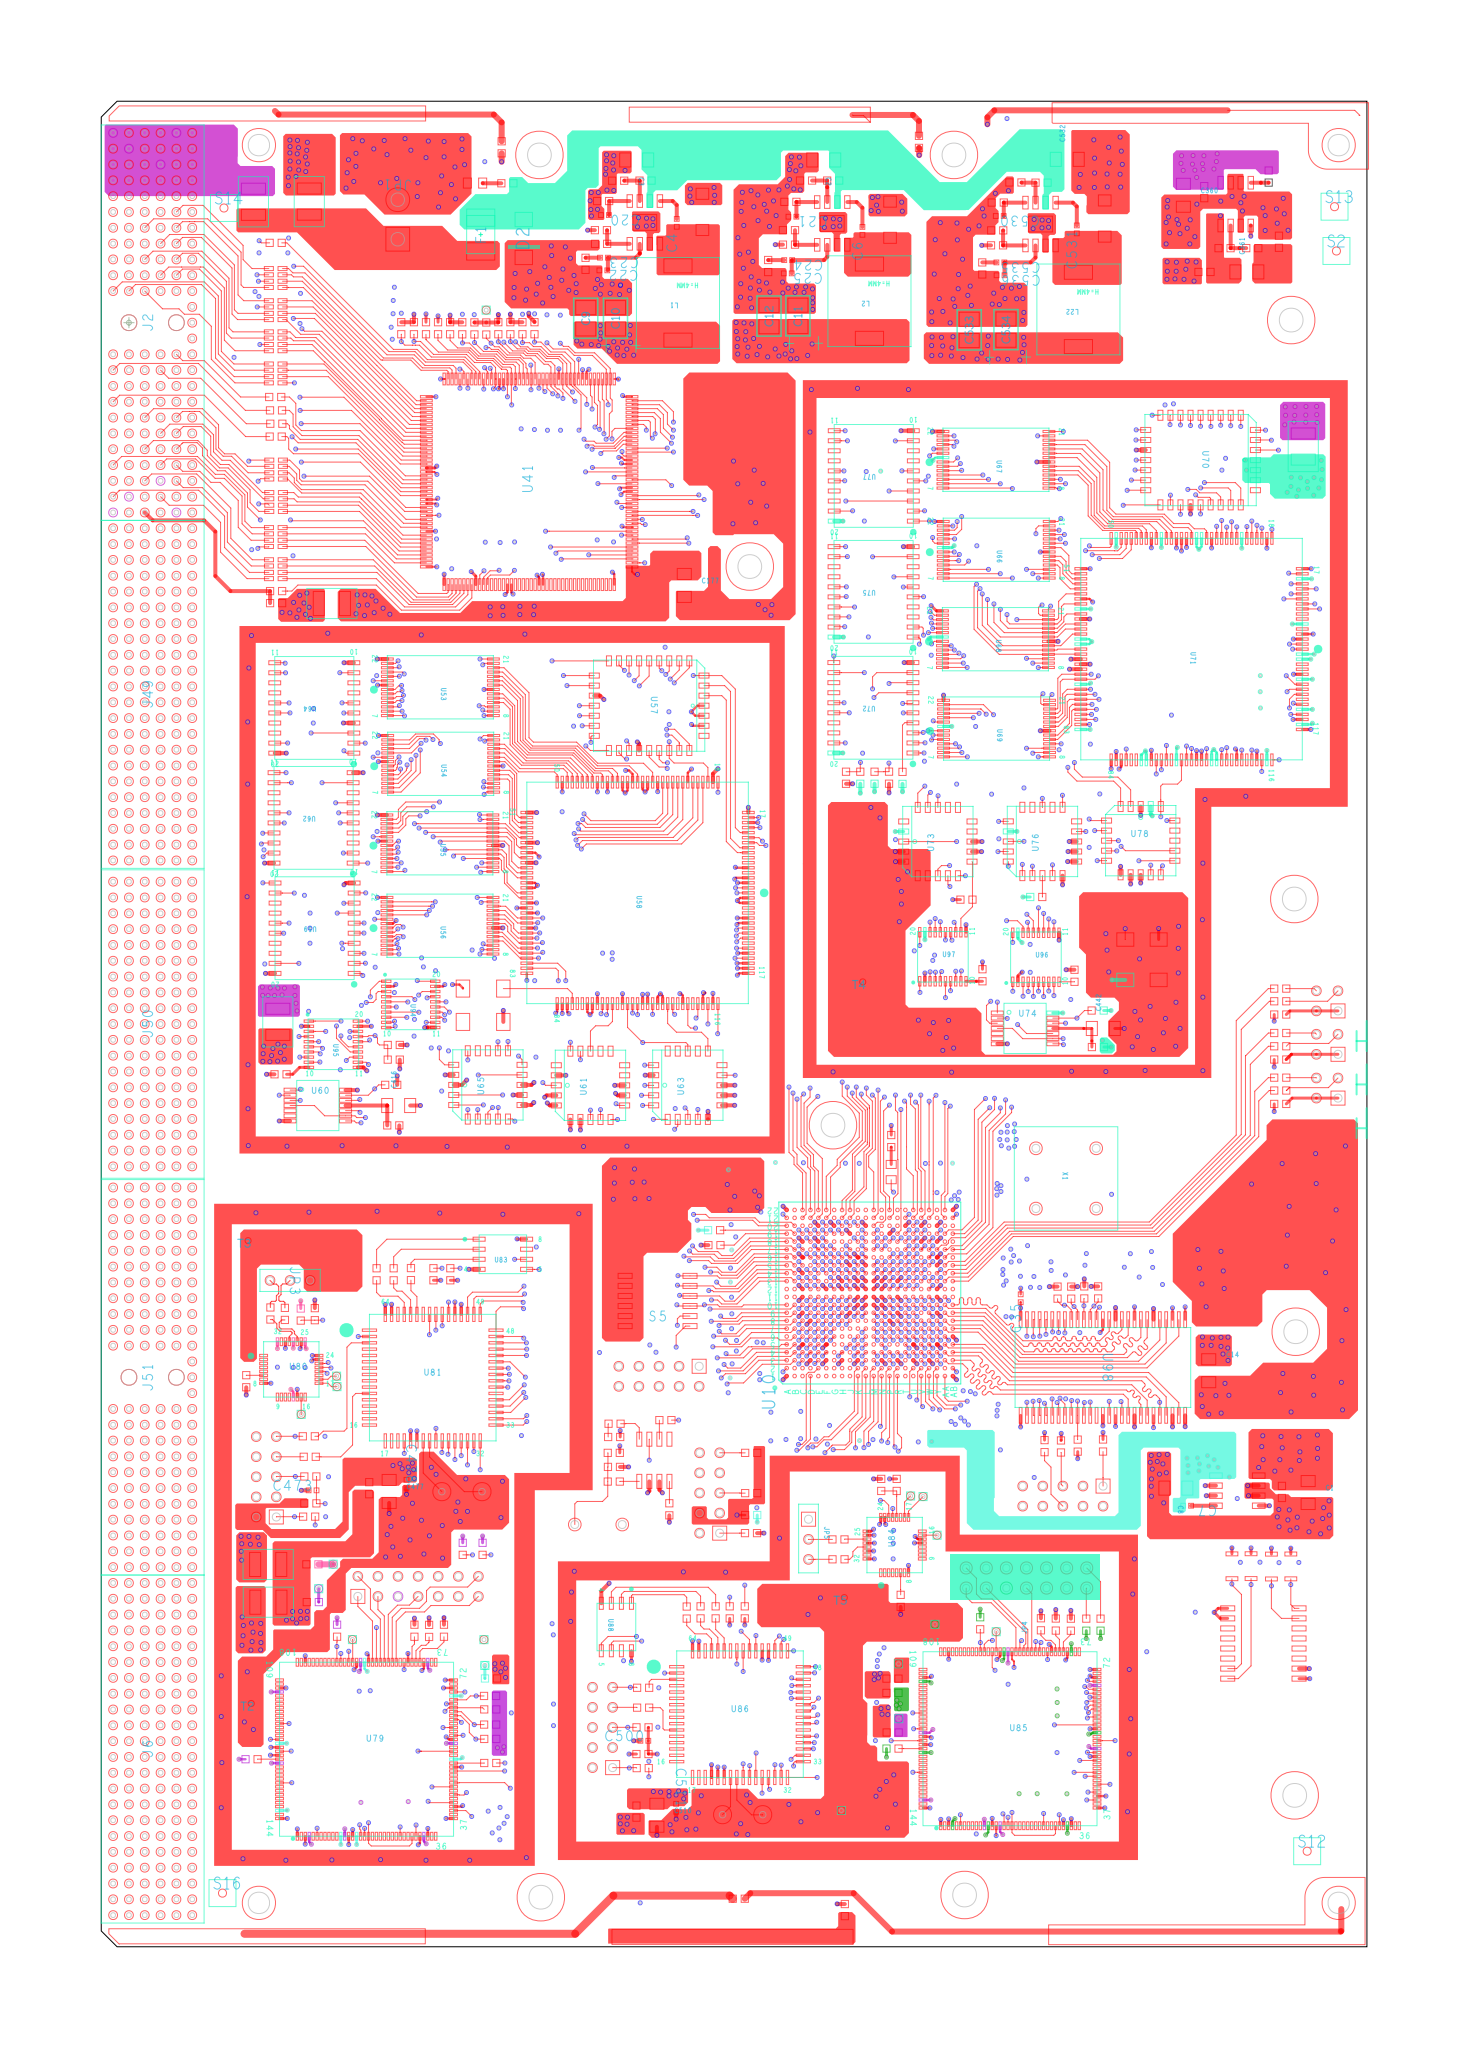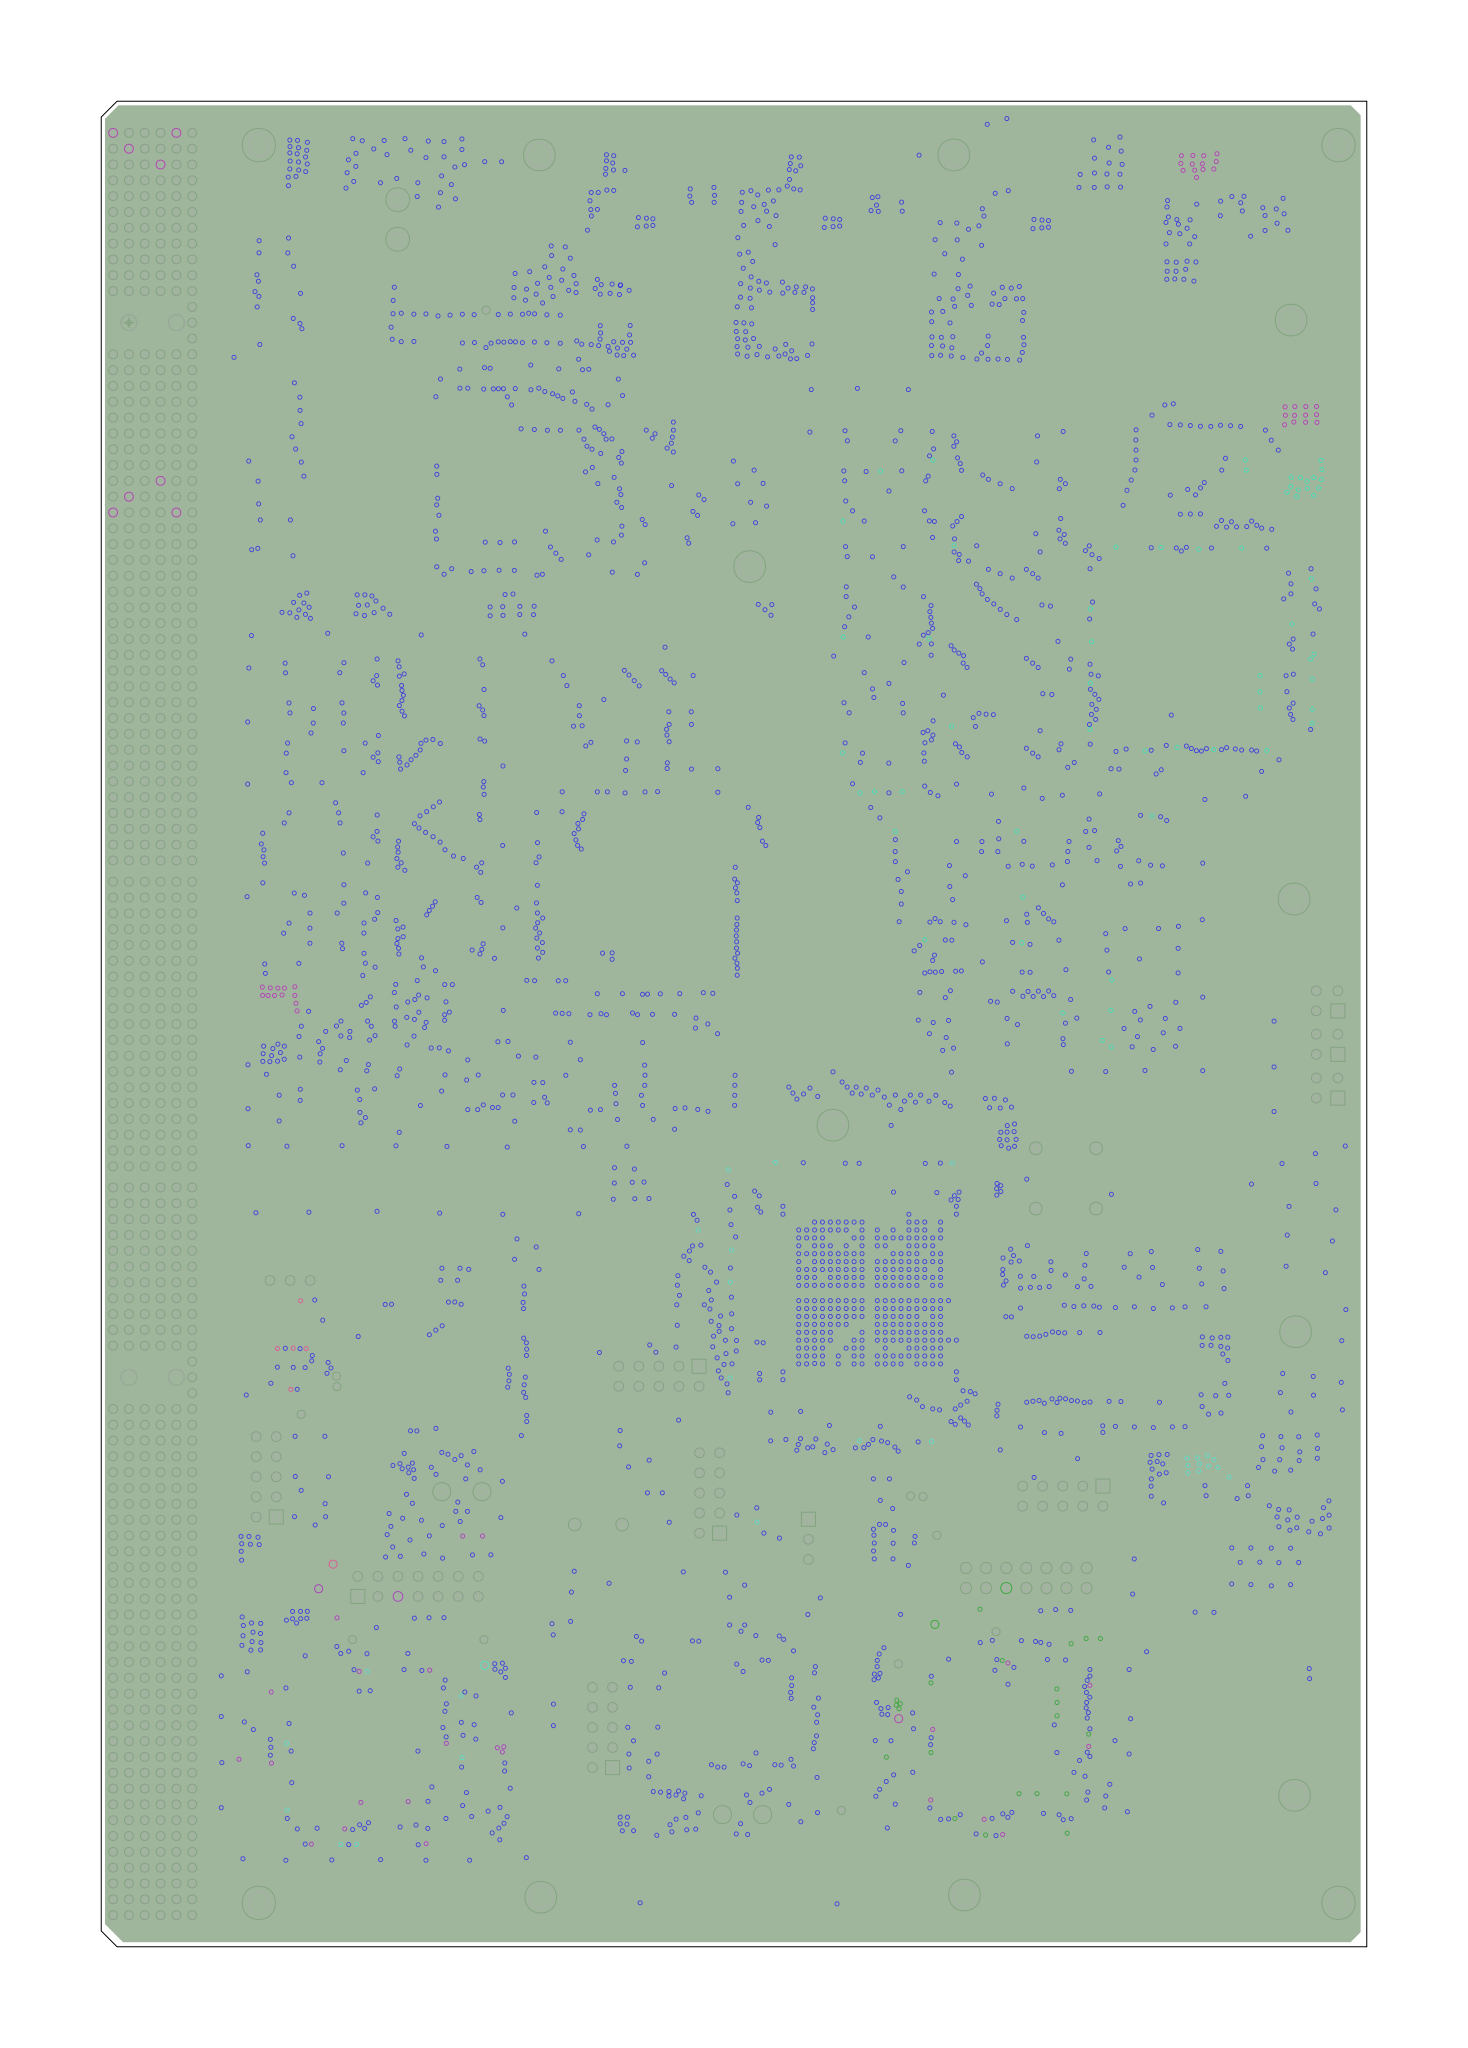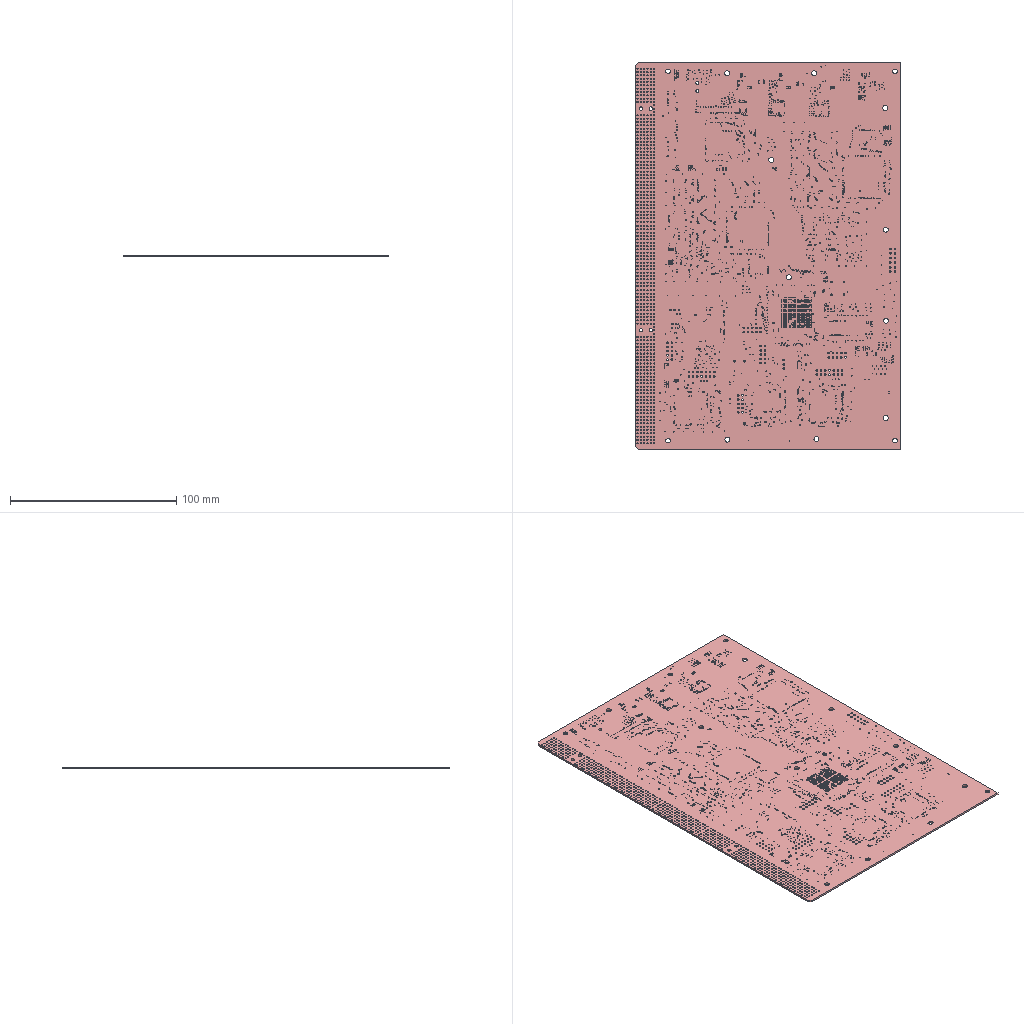Circuit board layout | Cadence Allegro | box 160 x 233.4 x 1.1 mm
Layer stack:
# Cadence Allegro layer stack of  (unit mm; from the constraint file cross-section; dielectric type: 0 not recorded (Allegro does not mark core vs prepreg), 3 surface material)
index,name,kind,layer,copper_thickness_mm,dielectric_type,dielectric_thickness_mm,dielectric_material,dielectric_constant
0,Top Surface,other,,,,,,
1,TOP,copper,TOP,0.0483,,,,
2,Dielectric1,dielectric,,,0,0.1143,FR-4,4.5
3,GND2,copper,GND2,0.0305,,,,
4,Dielectric2,dielectric,,,0,0.254,FR-4,4.5
5,IN3,copper,IN3,0.0305,,,,
6,Dielectric3,dielectric,,,0,0.254,FR-4,4.5
7,IN4,copper,IN4,0.0305,,,,
8,Dielectric4,dielectric,,,0,0.254,FR-4,4.5
9,VCC5,copper,VCC5,0.0305,,,,
10,Dielectric5,dielectric,,,0,0.1143,FR-4,4.5
11,BOTTOM,copper,BOTTOM,0.0483,,,,
12,Bottom Surface,other,,,,,,
# drill layer pairs: low layer,high layer
drill_pair,TOP,BOTTOM
Part placement, first 524 of 690 lines:
REFDES,COMP_VALUE,SYM_NAME,SYM_X,SYM_Y,SYM_ROTATE,SYM_MIRROR
C1,10uF,16V,CP3216,5868.969,-5823.437,0.000,NO
C2,10uF,16V,CP3216,3458.000,810.000,270.000,NO
C3,10uF,16V,CP3216,2527.000,810.000,270.000,NO
C4,0.1uF,C0402,2726.500,497.000,90.000,NO
C5,0.1uF,C0402,4890.500,-4389.500,90.000,YES
C6,0.1uF,C0402,3650.500,457.000,90.000,NO
C7,0.1uF,C0402,5266.508,-5889.256,180.000,NO
C8,10uF,16V,CP3216,5210.500,-5801.500,270.000,NO
C9,47uF,CP3528,2273.500,22.000,180.000,NO
C10,47uF,CP3528,2421.500,22.000,180.000,NO
C11,47uF,CP3528,3329.500,34.000,180.000,NO
C12,47uF,CP3528,3185.500,33.000,180.000,NO
C14,10uF,16V,CP3216,5374.000,-5160.000,0.000,NO
C15,10uF,16V,CP3216,4272.000,-5367.000,0.000,YES
C16,0.1uF,C0402,4953.992,-4654.256,270.000,YES
C17,0.1uF,C0402,2616.500,-5791.500,180.000,YES
C18,1uF,C0603,2414.000,-5696.000,0.000,NO
C19,2.2uF,C0603,5738.500,-5820.500,90.000,NO
C20,0.015uF,C0402,2368.992,535.744,180.000,NO
C21,0.015uF,C0402,3302.000,527.500,180.000,NO
C22,10pF,C0402,2361.000,260.500,180.000,NO
C23,180pF,C0402,2364.000,323.500,180.000,NO
C24,180pF,C0402,3281.000,311.500,180.000,NO
C25,10pF,C0402,3279.000,245.500,180.000,NO
C26,10pF,C0402,5584.756,-6189.992,90.000,YES
C27,10pF,C0402,5686.350,-6192.276,90.000,YES
C28,10pF,C0402,5782.425,-6191.276,90.000,YES
C29,10pF,C0402,5489.126,-6190.673,90.000,YES
C30,1uF,C0603,3065.000,-4490.000,0.000,YES
C31,1uF,C0603,4285.008,-4607.256,180.000,YES
C32,0.1uF,C0402-BGA,3074.000,-4551.000,180.000,YES
C33,0.1uF,C0402-BGA,4101.000,-4438.000,90.000,YES
C35,0.1uF,C0402,4438.256,-4856.508,90.000,NO
C36,0.1uF,C0402-BGA,3273.677,-4436.559,90.000,YES
C37,0.1uF,C0402-BGA,3527.500,-4451.500,180.000,YES
C38,1uF,C0603,3058.000,-4290.000,0.000,YES
C39,0.1uF,C0402-BGA,4060.000,-4478.000,90.000,YES
C40,0.1uF,C0402-BGA,3982.500,-4476.500,90.000,YES
C41,0.1uF,C0402-BGA,3629.500,-4477.500,90.000,YES
C42,0.1uF,C0402-BGA,3431.000,-4477.000,90.000,YES
C43,1uF,C0603,4286.000,-4789.000,180.000,YES
C46,0.1uF,C0402-BGA,3865.000,-4515.000,90.000,YES
C47,0.1uF,C0402-BGA,4001.000,-4575.000,0.000,YES
C48,0.1uF,C0402-BGA,3527.000,-4553.000,0.000,YES
C49,0.1uF,C0402-BGA,3067.331,-4349.157,180.000,YES
C50,0.1uF,C0402-BGA,4276.000,-4845.000,0.000,YES
C51,0.1uF,C0402-BGA,4274.756,-4660.992,0.000,YES
C54,0.1uF,C0402-BGA,3786.000,-4555.000,90.000,YES
C55,0.1uF,C0402-BGA,3335.000,-4811.500,180.000,YES
C56,0.1uF,C0402-BGA,3531.000,-4772.000,180.000,YES
C57,0.1uF,C0402,5352.732,-6419.051,180.000,YES
C58,0.1uF,C0402-BGA,3752.000,-4834.000,180.000,YES
C59,0.1uF,C0402-BGA,3332.909,-4614.713,180.000,YES
C60,0.1uF,C0402-BGA,4003.000,-4653.000,0.000,YES
C61,0.1uF,C0402-BGA,3608.323,-4653.094,0.000,YES
C62,0.1uF,C0402-BGA,3756.000,-4650.000,0.000,YES
C63,0.001uF,C0402,3684.756,-4696.992,90.000,YES
C64,0.1uF,C0402-BGA,3623.500,-4829.000,0.000,YES
C65,0.1uF,C0402-BGA,3609.000,-4732.000,0.000,YES
C66,0.1uF,C0402-BGA,3533.000,-4836.000,0.000,YES
C67,0.1uF,C0402-BGA,3353.000,-4713.000,270.000,YES
C68,0.1uF,C0402-BGA,4021.000,-4752.000,270.000,YES
C69,0.1uF,C0402-BGA,3785.000,-4753.000,270.000,YES
C70,0.1uF,C0402-BGA,3746.000,-4752.000,270.000,YES
C71,0.1uF,C0402-BGA,3823.000,-4753.000,270.000,YES
C72,0.1uF,C0402-BGA,3413.000,-4771.000,0.000,YES
C73,0.1uF,C0402-BGA,4042.000,-4828.000,0.000,YES
C74,0.1uF,C0402-BGA,3372.102,-4849.945,180.000,YES
C75,0.1uF,C0402-BGA,4040.000,-4888.000,0.000,YES
C76,0.1uF,C0402,5835.051,-6723.268,90.000,YES
C77,0.1uF,C0402-BGA,3837.500,-4829.500,0.000,YES
C78,0.1uF,C0402-BGA,3824.858,-4909.000,270.000,YES
C79,0.1uF,C0402-BGA,3588.638,-4909.000,270.000,YES
C80,0.1uF,C0402-BGA,3708.756,-4909.992,90.000,YES
C81,0.1uF,C0402-BGA,3668.756,-4909.992,90.000,YES
C82,0.1uF,C0402-BGA,3628.756,-4911.992,90.000,YES
C83,0.1uF,C0402-BGA,3373.000,-4928.000,180.000,YES
C84,0.1uF,C0402-BGA,4002.000,-4929.000,0.000,YES
C85,0.1uF,C0402-BGA,3843.756,-4966.992,0.000,YES
C86,0.1uF,C0402,5312.492,-4898.744,180.000,YES
C87,0.1uF,C0402,5143.992,-5462.744,180.000,YES
C88,0.1uF,C0402-BGA,3843.756,-5006.992,180.000,YES
C89,0.1uF,C0402-BGA,3411.000,-4968.000,180.000,YES
C90,0.1uF,C0402-BGA,3075.000,-5119.000,180.000,YES
C91,0.1uF,C0402-BGA,3412.500,-5086.000,0.000,YES
C92,0.1uF,C0402,4960.256,-4899.992,0.000,YES
C93,0.1uF,C0402,4789.244,-5027.508,0.000,YES
C94,0.1uF,C0402-BGA,3353.000,-5183.000,270.000,YES
C95,0.1uF,C0402-BGA,4081.000,-5047.000,0.000,YES
C96,0.1uF,C0402-BGA,3077.520,-5066.528,180.000,YES
C97,0.1uF,C0402-BGA,3961.476,-5086.335,180.000,YES
C98,0.1uF,C0402-BGA,4235.000,-4904.500,0.000,YES
C99,0.1uF,C0402,4955.756,-5462.492,180.000,YES
C100,0.1uF,C0402,5148.256,-4906.992,0.000,YES
C101,0.1uF,C0402-BGA,3903.598,-5145.220,270.000,YES
C102,0.1uF,C0402-BGA,3746.118,-5145.220,270.000,YES
C103,0.1uF,C0402-BGA,3681.000,-5155.000,270.000,YES
C104,0.1uF,C0402-BGA,3509.898,-5145.220,270.000,YES
C105,0.1uF,C0402-BGA,3470.528,-5145.220,270.000,YES
C106,1uF,C0603,3068.000,-5008.000,0.000,YES
C107,0.1uF,C0402-BGA,4100.000,-5224.000,270.000,YES
C108,0.1uF,C0402-BGA,4020.500,-5185.000,270.000,YES
C109,0.1uF,C0402-BGA,3825.000,-5146.000,270.000,YES
C110,0.1uF,C0402-BGA,3273.677,-5223.961,270.000,YES
C111,0.1uF,C0402-BGA,4232.500,-5084.000,0.000,YES
C112,1uF,C0603,4242.492,-5144.244,180.000,YES
C113,1uF,C0603,4244.992,-4959.244,180.000,YES
C114,1uF,C0603,3065.000,-5183.000,0.000,YES
C165,0.1uF,C0402,1490.000,-735.500,270.000,YES
C166,0.1uF,C0402,1496.500,-891.000,270.000,YES
C167,0.1uF,C0402,1490.000,-1057.000,90.000,YES
C168,0.1uF,C0402,1892.000,-1302.000,0.000,YES
C169,0.1uF,C0402,2052.000,-1302.000,0.000,YES
C170,0.1uF,C0402,2482.000,-1252.000,0.000,YES
C171,0.1uF,C0402,2502.000,-832.000,90.000,YES
C172,0.1uF,C0402,2502.000,-692.000,90.000,YES
C173,0.1uF,C0402,2470.000,-307.000,90.000,YES
C174,0.1uF,C0402,2272.000,-279.638,180.000,YES
C175,0.1uF,C0402,1852.000,-282.000,180.000,YES
C176,0.1uF,C0402,1519.000,-306.138,270.000,YES
C177,10uF,16V,CP3216,2764.000,-1308.000,0.000,NO
C358,0.1uF,C0402,5501.500,491.500,0.000,YES
C359,2.2uF,C0603,5351.815,649.787,90.000,NO
C360,10uF,16V,CP3216,5248.012,634.110,0.000,NO
C361,10uF,16V,CP3216,5563.890,252.732,90.000,NO
C416,4.7uF,CP3216,1342.465,-3896.969,90.000,NO
C417,0.1uF,C0402,3068.102,-2841.268,90.000,YES
C418,0.1uF,C0402,2855.732,-2253.102,0.000,YES
C419,0.1uF,C0402,2597.232,-2298.602,0.000,YES
C420,0.1uF,C0402,3066.898,-3161.732,270.000,YES
C421,0.1uF,C0402,3068.602,-2981.268,90.000,YES
C422,0.1uF,C0402,2750.268,-1999.898,180.000,YES
C423,0.1uF,C0402,3082.602,-2471.268,90.000,YES
C424,0.1uF,C0402,721.000,-2663.500,90.000,YES
C425,0.1uF,C0402,1983.102,-2969.768,90.000,YES
C426,0.1uF,C0402,2885.268,-3378.898,180.000,YES
C427,0.1uF,C0402,2626.768,-3381.398,180.000,YES
C428,0.1uF,C0402,2394.768,-3339.398,180.000,YES
C429,0.1uF,C0402,2235.268,-3403.898,180.000,YES
C430,0.1uF,C0402,1999.732,-3234.602,0.000,YES
C431,0.1uF,C0402,1284.102,-1786.268,90.000,YES
C432,0.1uF,C0402,1283.602,-2956.268,90.000,YES
C433,0.1uF,C0402,3077.898,-2737.732,270.000,YES
C434,0.1uF,C0402,1289.102,-2165.268,90.000,YES
C435,0.1uF,C0402,1280.102,-2559.268,90.000,YES
C436,0.1uF,C0402,2425.732,-2305.102,0.000,YES
C437,0.1uF,C0402,2750.268,-1936.898,180.000,YES
C438,0.1uF,C0402,716.000,-3212.000,90.000,YES
C439,0.1uF,C0402,2155.898,-2391.732,270.000,YES
C440,0.1uF,C0402,1993.602,-2614.768,90.000,YES
C441,0.1uF,C0402,1990.398,-2844.232,270.000,YES
C442,4.7uF,CP3216,4849.465,-3513.488,90.000,NO
C443,0.1uF,C0402,5600.232,-1124.102,0.000,YES
C444,0.1uF,C0402,5848.102,-1247.268,90.000,YES
C445,0.1uF,C0402,3611.500,-1564.500,0.000,YES
C446,0.1uF,C0402,3602.000,-987.500,0.000,YES
C447,0.1uF,C0402,4687.390,-3416.807,90.000,YES
C448,0.1uF,C0402,5498.307,-675.110,180.000,YES
C449,0.1uF,C0402,5266.732,-2163.602,0.000,YES
C450,0.1uF,C0402,4167.232,-2010.102,0.000,YES
C451,0.1uF,C0402,3965.898,-1635.732,270.000,YES
C452,0.1uF,C0402,4155.232,-1110.602,0.000,YES
C453,0.1uF,C0402,3978.398,-724.232,270.000,YES
C454,0.1uF,C0402,5498.268,-733.898,180.000,YES
C455,0.1uF,C0402,4850.602,-3251.768,90.000,YES
C456,0.1uF,C0402,3855.898,-2553.732,270.000,YES
C457,0.1uF,C0402,4374.898,-2549.732,270.000,YES
C458,0.1uF,C0402,5073.732,-2170.102,0.000,YES
C459,0.1uF,C0402,4744.898,-2054.232,270.000,YES
C460,0.1uF,C0402,4732.602,-1757.768,90.000,YES
C461,0.1uF,C0402,4792.102,-1519.268,90.000,YES
C462,0.1uF,C0402,5356.732,-1085.102,0.000,YES
C463,0.1uF,C0402,3601.000,-2143.000,0.000,YES
C464,0.1uF,C0402,5060.268,-2406.898,180.000,YES
C465,0.1uF,C0402,5461.732,-2164.102,0.000,YES
C466,0.1uF,C0402,5637.768,-2168.898,180.000,YES
C467,0.1uF,C0402,4751.602,-1399.268,90.000,YES
C468,0.1uF,C0402,1291.067,-4927.528,0.000,YES
C469,0.1uF,C0402,1639.933,-4933.472,180.000,YES
C470,0.1uF,C0402,1982.000,-4581.500,270.000,YES
C471,1uF,C0603,704.110,-4932.268,270.000,NO
C472,1uF,C0603,776.110,-4934.268,270.000,NO
C473,0.1uF,C0402,913.933,-5812.528,0.000,NO
C474,0.1uF,C0402,1416.567,-5554.528,0.000,YES
C475,22pF,C0402,1577.000,-5917.000,0.000,YES
C476,22pF,C0402,1737.894,-5917.472,180.000,YES
C477,10uF,16V,CP3216,1295.138,-5818.102,0.000,NO
C478,0.1uF,C0402,1381.472,-5779.894,270.000,NO
C479,0.1uF,C0402,749.890,-7093.059,90.000,YES
C480,0.1uF,C0402,1200.890,-6763.059,90.000,YES
C481,0.1uF,C0402,1615.890,-7168.059,90.000,YES
C482,0.1uF,C0402,753.102,-7424.268,90.000,YES
C483,0.1uF,C0402,1106.232,-7542.602,0.000,YES
C484,0.1uF,C0402,1616.898,-6811.732,270.000,YES
C485,0.1uF,C0402,1477.732,-6672.102,0.000,YES
C486,0.1uF,C0402,1459.732,-7535.102,0.000,YES
C487,0.1uF,C0402,1146.102,-6762.268,90.000,YES
C488,0.1uF,C0402,1617.898,-7062.732,270.000,YES
C489,0.1uF,C0402,864.232,-7533.602,0.000,YES
C490,0.1uF,C0402,745.898,-6808.732,270.000,YES
C491,0.1uF,C0402,877.102,-5154.268,90.000,YES
C492,0.1uF,C0402,818.102,-5153.268,90.000,YES
C493,0.1uF,C0402,738.890,-5153.307,90.000,YES
C494,0.1uF,C0402,828.268,-5348.898,180.000,YES
C495,0.1uF,C0402,2819.287,-6601.378,0.000,YES
C496,0.1uF,C0402,3165.650,-6622.323,180.000,YES
C497,1uF,C0603,3531.598,-6155.890,0.000,NO
C498,1uF,C0603,3531.307,-6056.890,0.000,NO
C499,0.1uF,C0402,2481.433,-6630.972,180.000,YES
C500,0.1uF,C0402,2565.150,-7059.378,0.000,NO
C501,0.1uF,C0402,4335.732,-7482.102,0.000,YES
C502,0.1uF,C0402,3950.102,-7375.268,90.000,YES
C503,0.1uF,C0402,4820.102,-7118.268,90.000,YES
C504,0.1uF,C0402,4820.898,-6758.732,270.000,YES
C505,0.1uF,C0402,3953.102,-7027.268,90.000,YES
C506,0.1uF,C0402,4375.602,-6730.268,90.000,YES
C507,0.1uF,C0402,2947.720,-7229.850,0.000,YES
C508,22pF,C0402,2973.000,-7523.000,0.000,YES
C509,22pF,C0402,3135.000,-7526.000,180.000,YES
C510,10uF,16V,CP3216,2627.657,-7430.102,0.000,NO
C511,0.1uF,C0402,2723.472,-7392.933,270.000,NO
C512,0.1uF,C0402,4652.732,-7482.102,0.000,YES
C513,0.1uF,C0402,4079.732,-7483.102,0.000,YES
C514,0.1uF,C0402,4821.898,-7009.732,270.000,YES
C515,0.1uF,C0402,4674.732,-6616.102,0.000,YES
C516,0.1uF,C0402,3952.398,-6752.232,270.000,YES
C517,0.1uF,C0402,4236.732,-7483.102,0.000,YES
C518,0.1uF,C0402,3754.268,-6153.898,180.000,YES
C519,0.1uF,C0402,3755.268,-6075.898,180.000,YES
C520,0.1uF,C0402,3947.898,-6061.732,270.000,YES
C521,0.1uF,C0402,3756.268,-6011.898,180.000,YES
C526,0.1uF,C0402,1526.000,-3284.000,90.000,YES
C527,0.1uF,C0402,1279.500,-3324.500,90.000,YES
C530,0.015uF,C0402,4334.000,531.000,180.000,NO
C531,0.1uF,C0402,4717.500,464.500,90.000,NO
C532,10uF,16V,CP3216,4670.000,813.000,90.000,NO
C533,47uF,CP3528,4182.000,-36.000,180.000,NO
C534,47uF,CP3528,4365.000,-34.500,180.000,NO
C535,180pF,C0402,4337.000,300.000,180.000,NO
C536,10pF,C0402,4338.000,236.000,180.000,NO
C537,0.1uF,C0402,1141.500,-3522.000,270.000,YES
C538,0.1uF,C0402,894.500,-3482.500,270.000,YES
C539,0.1uF,C0402,3990.000,-3110.000,0.000,YES
C540,0.1uF,C0402,4466.000,-3200.000,180.000,YES
C541,0.1uF,C0402,4465.500,-3125.000,0.000,YES
C542,0.1uF,C0402,3981.000,-3194.500,180.000,YES
D1,Red_LED,D0805,1722.449,694.925,90.000,NO
D2,SMBJ12VA,DO214AA,1965.098,419.075,90.000,NO
D3,B320A,B320A,2854.000,551.500,270.000,NO
D4,B320A,B320A,3788.000,512.500,270.000,NO
D5,1N4148,LL34,5489.524,-6190.673,0.000,NO
D6,1N4148,LL34,5782.598,-6191.276,0.000,NO
D7,1N4148,LL34,5686.126,-6191.874,0.000,NO
D8,1N4148,LL34,5584.756,-6189.992,0.000,NO
D9,LED_D,LED_DL,6010.000,-3426.000,90.000,NO
D10,Red_LED,D0805,3793.748,-4228.291,180.000,NO
D11,LED_D,LED_DL,6010.000,-3642.000,90.000,NO
D12,LED_D,LED_DL,6010.000,-3860.000,90.000,NO
D15,Red_LED,D0805,1692.421,-1161.362,180.000,YES
D16,B320A,B320A,4856.500,518.500,270.000,NO
F1,PPTC 24V  1.5A/3.0A,MF-MSMF150/24X,F1812,1750.776,438.575,90.000,NO
F6,BLM18PG300SN1,F0603,5723.602,402.807,90.000,NO
J2,CompactPCI-J1,CPCI_J1_4,118.110,0.000,90.000,NO
J6,CPCI_AB110_J5,CPCI_J2_5,118.110,-7100.394,90.000,NO
J49,CPCI_AB110_J2,CPCI_J2_5,118.110,-1850.240,90.000,NO
J50,CPCI_AB95_J3,CPCI_J3,118.110,-3491.339,90.000,NO
J51,CPCI_A110_J4,CPCI_J1_4,118.110,-5249.882,90.000,NO
JP1,HEADER 2,POWER_2_B,1337.874,710.598,180.000,NO
JP2,HEADER 7X2,ZIP14,1139.228,-6340.701,0.000,NO
JP3,HEADER 3,SIP3,802.110,-4767.598,270.000,NO
JP4,HEADER 7X2,SIP14_254,5067.000,-6299.000,90.000,NO
JP5,HEADER 3,ZIP3,3382.228,-6056.370,270.000,NO
L1,2.5uH,MSS1038,2732.500,98.000,180.000,NO
L2,2.5uH,MSS1038,3685.500,107.000,180.000,NO
L3,BLM18PG300SN1,F0603,5730.000,-3444.000,0.000,NO
L4,BLM18PG300SN1,F0603,5730.000,-3668.000,0.000,NO
L5,BLM18PG300SN1,F0603,5730.000,-3889.000,0.000,NO
L6,BLM18PG300SN1,L0603,3064.000,-4417.000,0.000,YES
L7,BLM18PG300SN1,L0603,4284.508,-4542.256,180.000,YES
L8,BLM18PG300SN1,L0603,3057.756,-4216.992,0.000,YES
L9,BLM18PG300SN1,L0603,4285.000,-4721.000,180.000,YES
L10,BLM18PG300SN1,L0603,3067.000,-4934.000,0.000,YES
L11,BLM18PG300SN1,L0603,4241.500,-5211.500,180.000,YES
L12,BLM18PG300SN1,L0603,4244.500,-5027.000,180.000,YES
L13,BLM18PG300SN1,L0603,3065.000,-5253.000,0.000,YES
L14,BLM18PG300SN1,F0603,1195.890,-5801.941,90.000,NO
L15,BLM18PG300SN1,F0603,1801.941,-6749.110,180.000,NO
L16,BLM18PG300SN1,F0603,915.059,-6368.890,0.000,NO
L17,BLM18PG300SN1,F0603,913.059,-6180.890,0.000,NO
L18,BLM18PG300SN1,F0603,3801.059,-7017.890,0.000,NO
L19,BLM18PG300SN1,F0603,2525.890,-7411.941,90.000,NO
L20,BLM18PG300SN1,F0603,3800.059,-6820.890,0.000,NO
L21,BLM18PG300SN1,F0603,3800.059,-6749.890,0.000,NO
L22,2.5uH,MSS1038,4725.500,66.000,180.000,NO
R1,10M,R0603,3932.000,900.000,90.000,NO
R2,10M,R0603,1855.000,873.000,90.000,NO
R3,500R,R0603,1883.449,693.925,0.000,NO
R10,4.7K,R0603,2647.000,-4698.000,0.000,YES
R11,4.7K,R0603,2647.000,-4766.000,0.000,YES
R12,4.7K,R0603,2646.000,-4835.000,0.000,YES
R13,4.7K,R0603,2646.000,-4904.000,0.000,YES
R14,33R,R0603,4514.500,-4293.500,270.000,YES
R15,4.7K,R0603,2647.000,-4974.000,0.000,YES
R16,4.7K,R0603,2648.000,-5045.000,0.000,YES
R17,200R,R0603,5730.000,-3315.000,0.000,NO
R18,200R,R0603,5730.000,-3378.000,0.000,NO
R19,200R,R0603,5730.000,-3536.000,0.000,NO
R20,33R,R0603,4502.055,-4705.244,0.000,YES
R21,200R,R0603,5730.000,-3602.000,0.000,NO
R22,200R,R0603,5730.000,-3758.268,0.000,NO
R23,200R,R0603,5730.000,-3822.268,0.000,NO
R24,27K,R0603,2689.500,-5907.000,270.000,NO
R25,NU_0R,R0603,2670.000,-5463.000,0.000,NO
R26,10K,R0603,2413.000,-5626.000,180.000,NO
R27,NU_0R,R0603,2417.000,-5481.000,180.000,NO
R28,10K,R0603,2415.000,-5547.000,0.000,NO
R29,33R,R0603,2413.000,-5769.000,180.000,NO
R42,10M,R0603,3035.000,-7845.500,180.000,NO
R43,10M,R0603,3563.000,-7902.000,270.000,NO
R44,10M,R0603,3933.000,901.000,270.000,YES
R45,10M,R0603,1771.000,873.000,270.000,YES
R46,150K,R0603,2571.008,707.256,180.000,NO
R47,48.7K,R0603,2434.992,706.744,180.000,NO
R48,150K,R0603,3505.000,707.500,180.000,NO
R49,48.7K,R0603,3370.000,707.500,180.000,NO
R50,1M,R0603,2360.000,605.500,180.000,NO
R51,1M,R0603,3292.000,601.500,180.000,NO
R52,0R,R0603,5622.500,-5860.500,270.000,YES
R53,1K,R0603,5446.500,-5853.500,180.000,YES
R54,1.07K,R0603,5446.500,-5793.500,0.000,YES
R55,10.2K,R0603,2349.000,460.500,0.000,NO
R56,20.4K,R0603,2350.000,392.500,180.000,NO
R57,75K,R0603,2272.500,293.000,270.000,NO
R58,10.2K,R0603,3285.000,388.500,0.000,NO
R59,3.24K,R0603,3285.000,460.500,180.000,NO
R60,75K,R0603,3181.500,282.000,270.000,NO
R61,0R,R0603,3282.551,-4254.268,270.000,YES
R62,NU_0R,R0603,3217.551,-4253.268,270.000,YES
R63,49.9R,R0603,2912.268,-4517.551,180.000,NO
R64,0R,R0603,4280.976,-4396.925,180.000,YES
R69,10K,R0603,3963.756,-4255.992,270.000,YES
R70,NU_0R,R0603,3889.756,-4255.992,90.000,YES
R71,NU_0R,R0603,3703.756,-4255.992,90.000,YES
R72,10K,R0603,3634.756,-4255.992,270.000,YES
R73,NU_0R,R0603,3565.756,-4254.992,270.000,YES
R74,10K,R0603,3497.756,-4254.992,90.000,YES
R75,NU_0R,R0603,3427.756,-4254.992,90.000,YES
R76,10K,R0603,3356.756,-4254.992,270.000,YES
R77,0R,R0603,3097.000,-5935.500,180.000,NO
R78,NU_0R,R0603,3095.000,-5935.500,0.000,YES
R79,10K,R0603,3097.000,-5826.500,180.000,NO
R80,10K,R0603,3096.000,-6025.500,180.000,NO
R81,10K,R0603,3097.000,-5626.000,180.000,NO
R82,NU_0R,R0603,4281.000,-4463.000,180.000,YES
R83,49.9R,R0603,2914.000,-4592.000,180.000,NO
R84,NU_0R,R0603,3069.000,-4616.000,0.000,YES
R85,49.9R,R0603,4039.000,-4259.000,270.000,YES
R86,0R,R0603,3069.000,-4706.000,0.000,YES
R87,49.9R,R0603,4099.000,-4259.000,270.000,YES
R90,200R,R0603,3794.000,-4074.000,90.000,NO
R91,NU_0R,R0603,3343.000,-5492.500,90.000,YES
R92,NU_0R,R0603,3194.268,-5492.949,90.000,YES
R93,NU_0R,R0603,3065.000,-4776.000,0.000,YES
R96,0R,R0603,3066.000,-4851.000,0.000,YES
R97,10K,R0603,4638.701,-5594.185,90.000,NO
R98,10K,R0603,4557.000,-5592.500,270.000,NO
R105,0R,R0603,3703.000,-5496.500,90.000,YES
R106,NU_0R,R0603,3636.000,-5496.500,90.000,YES
R107,10K,R0603,4848.000,-5589.500,90.000,NO
R108,10K,R0603,3419.000,-5491.500,270.000,YES
R109,NU_0R,R0603,3270.000,-5491.500,90.000,YES
R110,49.9R,R0603,3928.500,-5500.500,90.000,YES
R111,NU_0R,R0603,3064.000,-5387.000,0.000,YES
R112,0R,R0603,3064.000,-5327.000,0.000,YES
R113,49.9R,R0603,3995.000,-5501.000,90.000,YES
R114,10M,R0603,3036.000,-7915.000,0.000,YES
R115,10M,R0603,2511.500,-7896.000,90.000,YES
R159,NU_10R,R0603,493.000,-127.000,180.000,YES
R160,10R,R0603,732.421,-1336.138,0.000,NO
R161,10R,R0603,730.421,-436.638,180.000,YES
R162,10R,R0603,732.421,-502.638,180.000,YES
R163,10R,R0603,728.000,-370.000,0.000,NO
R164,10R,R0603,732.000,-436.500,0.000,NO
R165,10R,R0603,730.500,-567.000,0.000,NO
R166,10R,R0603,733.421,-628.638,180.000,YES
R167,10R,R0603,731.421,-567.138,180.000,YES
R168,10R,R0603,734.500,-694.000,180.000,YES
R169,10R,R0603,733.500,-503.000,0.000,NO
R170,10R,R0603,720.421,282.362,180.000,YES
R171,10R,R0603,725.421,-23.638,180.000,YES
R172,10R,R0603,730.421,-981.862,0.000,YES
R173,10R,R0603,730.421,397.362,0.000,NO
R174,10R,R0603,735.421,-762.638,0.000,YES
R175,10R,R0603,729.421,-371.638,0.000,YES
R176,10R,R0603,721.421,44.362,0.000,YES
R177,5.1K,R0603,732.421,-1396.138,0.000,NO
R178,NU_0R,R0603,729.421,-1210.138,180.000,YES
R179,NU_0R,R0603,723.421,347.362,180.000,YES
R180,5.1K,R0603,729.421,-1142.138,0.000,YES
R181,NU_0R,R0603,723.421,421.362,0.000,YES
R182,NU_0R,R0603,729.421,-1338.138,180.000,YES
R183,NU_0R,R0603,729.421,-1288.138,180.000,YES
R184,4.7K,R0603,1898.500,-27.500,270.000,YES
R185,4.7K,R0603,1838.500,-28.000,270.000,YES
R186,4.7K,R0603,2148.000,-461.000,90.000,YES
R187,4.7K,R0603,1838.421,-27.638,90.000,NO
R188,4.7K,R0603,2147.000,-30.000,270.000,YES
R189,4.7K,R0603,1847.421,-1161.362,270.000,YES
R190,4.7K,R0603,1778.500,-29.000,90.000,NO
R191,4.7K,R0603,1773.421,-1161.362,270.000,YES
R192,4.7K,R0603,1418.421,-27.638,90.000,NO
R193,NU_4.7K,R0603,1418.579,-27.638,270.000,YES
R194,4.7K,R0603,1919.421,-1160.362,270.000,YES
R195,NU_4.7K,R0603,1355.421,-27.638,90.000,NO
R196,NU_4.7K,R0603,1355.579,-27.638,270.000,YES
R197,200R,R0603,1606.421,-1153.362,270.000,YES
R198,NU_4.7K,R0603,1659.000,-28.000,90.000,NO
R199,4.7K,R0603,1719.500,-28.500,90.000,NO
R200,4.7K,R0603,1659.500,-28.000,270.000,YES
R201,NU_4.7K,R0603,1718.500,-28.000,270.000,YES
R202,1K,R0603,1243.138,-82.579,180.000,YES
R203,1K,R0603,720.421,117.362,0.000,YES
R204,33R,R0603,1240.862,176.579,0.000,YES
R205,33R,R0603,1240.862,110.579,0.000,YES
R206,4.7K,R0603,1478.421,-27.638,90.000,NO
R207,33R,R0603,1241.862,44.579,0.000,YES
R208,4.7K,R0603,1952.000,-459.598,90.000,YES
R209,4.7K,R0603,2018.000,-461.000,90.000,YES
R210,NU_1K,R0603,1243.138,-22.579,0.000,YES
R211,1K,R0603,720.421,177.362,180.000,YES
R212,4.7K,R0603,1538.421,-27.638,90.000,NO
R213,4.7K,R0603,1598.421,-27.638,90.000,NO
R214,4.7K,R0603,2019.000,-28.000,270.000,YES
R215,4.7K,R0603,1958.421,-27.638,90.000,NO
R216,100R,R0603,1777.000,-29.000,90.000,YES
R217,4.7K,R0603,2352.000,-1162.000,270.000,YES
R218,NU_4.7K,R0603,2018.421,-27.638,90.000,NO
R219,NU_4.7K,R0603,1959.000,-28.500,270.000,YES
R220,NU_4.7K,R0603,2412.000,-1162.000,270.000,YES
R221,4.7K,R0603,1898.421,-27.638,90.000,NO
R222,4.7K,R0603,2080.402,-30.098,270.000,YES
R223,4.7K,R0603,2083.000,-461.000,90.000,YES
R233,10K,R0603,4722.000,-5590.000,270.000,NO
R234,33R,R0603,4715.000,-5317.000,180.000,YES
R247,10K,R0603,4754.701,-4827.382,90.000,NO
R248,10K,R0603,4823.701,-4827.382,90.000,NO
R256,10K,R0603,4689.701,-4828.382,90.000,NO
R257,10K,R0603,4621.701,-4828.382,90.000,NO
R308,NU_0R,R1210,897.598,602.799,270.000,NO
R309,NU_0R,R1210,1010.000,-1398.000,180.000,NO
R314,1.7K,R0603,5452.807,370.898,0.000,NO
R315,1K,R0603,5590.807,371.110,0.000,NO
R316,0R,R0603,5672.390,727.307,90.000,NO
R329,NU_0R,R0603,5353.000,252.500,0.000,NO
R330,0R,R1210,619.598,601.799,270.000,NO
R346,33R,R0603,4502.500,-4633.000,0.000,YES
R401,NU_4.7K,R0603,1318.000,-3668.500,0.000,NO
R402,4.7K,R0603,1318.000,-3595.500,0.000,NO
R403,NU_4.7K,R0603,969.000,-2939.000,0.000,YES
R404,4.7K,R0603,969.000,-3014.000,0.000,YES
R405,4.7K,R0603,969.000,-3089.000,0.000,YES
R406,4.7K,R0603,1305.268,-3794.102,0.000,NO
R407,120K,R0603,1315.598,-3995.890,0.000,NO
R408,4.7K,R0603,2465.102,-3866.268,90.000,YES
R409,NU_4.7K,R0603,993.000,-1921.000,0.000,YES
R410,4.7K,R0603,994.000,-1993.000,0.000,YES
R411,4.7K,R0603,2748.693,-3954.102,0.000,YES
R412,20K,R0603,2794.598,-3119.110,180.000,YES
R413,20K,R0603,2794.598,-3053.110,180.000,YES
R414,20K,R0603,2794.598,-2986.110,180.000,YES
R415,NU_4.7K,R0603,3783.000,-2265.000,270.000,NO
R416,4.7K,R0603,3710.898,-2265.307,270.000,NO
R417,NU_4.7K,R0603,3568.898,-2265.307,270.000,NO
R418,4.7K,R0603,3639.898,-2265.307,270.000,NO
R419,4.7K,R0603,3850.000,-2266.000,270.000,NO
R420,4.7K,R0603,4821.307,-3424.102,0.000,NO
R421,120K,R0603,4822.598,-3605.890,0.000,NO
R422,4.7K,R0603,4168.307,-2872.102,0.000,NO
R423,NU_4.7K,R0603,3669.398,-808.193,270.000,YES
R424,4.7K,R0603,3741.398,-808.193,270.000,YES
R425,4.7K,R0603,4515.693,-2858.898,180.000,NO
R426,20K,R0603,5695.598,-1918.110,180.000,YES
R427,20K,R0603,5696.598,-1837.110,180.000,YES
R428,20K,R0603,5696.307,-1757.110,180.000,YES
R429,10K,R0603,1797.307,-6836.102,0.000,NO
R430,10K,R0603,1798.307,-6903.102,0.000,NO
R431,10K,R0603,1798.307,-7050.102,0.000,NO
R432,1K,R0603,855.110,-4937.598,270.000,NO
R433,1K,R0603,925.110,-4935.598,270.000,NO
R434,10K,R0603,1191.000,-7396.000,270.000,YES
R435,1K,R0603,1420.890,-6511.402,90.000,NO
R436,1K,R0603,1493.890,-6512.402,90.000,NO
R437,1K,R0603,1567.890,-6511.402,90.000,NO
R438,100K,R0603,583.890,-5269.402,90.000,NO
R439,1K,R0603,895.268,-5543.528,0.000,NO
R440,1K,R0603,896.894,-5943.528,0.000,NO
R441,10K,R0603,1429.000,-7392.000,90.000,YES
R442,10K,R0603,1035.898,-6511.307,270.000,NO
R443,10K,R0603,1797.732,-6978.685,180.000,NO
R444,0R,R0603,1798.307,-7169.890,0.000,NO
R445,4.7K,R0603,610.307,-7151.102,0.000,NO
R446,10K,R0603,1760.102,-6103.693,90.000,NO
R447,1K,R0603,899.894,-5645.528,0.000,NO
R448,10K,R0603,1661.315,-6103.732,90.000,NO
R449,4.7K,R0603,903.067,-5877.472,180.000,NO
R450,1K,R0603,902.894,-5743.528,0.000,NO
R451,4.7K,R0603,1515.472,-4736.933,270.000,NO
R452,4.7K,R0603,1599.472,-4736.933,270.000,NO
R453,100K,R0603,1232.528,-4737.106,90.000,NO
R454,100K,R0603,1317.528,-4737.106,90.000,NO
R455,100K,R0603,1403.528,-4736.106,90.000,NO
R456,10K,R0603,4685.732,-6801.315,0.000,YES
R457,10K,R0603,4553.185,-7352.732,270.000,YES
R458,10K,R0603,4688.693,-6935.102,0.000,YES
R459,1K,R0603,3821.110,-5785.598,270.000,NO
R460,1K,R0603,3744.110,-5785.598,270.000,NO
R461,10K,R0603,4395.685,-7352.732,270.000,YES
R462,1K,R0603,4538.890,-6479.402,90.000,NO
R463,1K,R0603,4612.890,-6480.732,90.000,NO
R464,1K,R0603,4687.890,-6481.402,90.000,NO
R465,100K,R0603,3840.890,-6362.732,90.000,NO
R466,10K,R0603,4631.102,-7353.307,90.000,YES
R467,10K,R0603,4236.685,-6474.268,270.000,NO
Pad and via stacks, first 110 of 114 lines:
# Allegro (Cadence) via spans and padstacks; design units: ("mils" 3 1000)
# via spans: padstack,start_layer,end_layer,net_example,count
VIA_10_20MIL,ETCH/TOP,ETCH/BOTTOM,DGND,2657
# Allegro padstack definitions: name,start_layer,end_layer,drill,plating,holeType,type
SMD95X100,"ETCH/TOP","ETCH/TOP",0.0,"PLATED","none","smd"
RX0_40Y1_00,"ETCH/TOP","ETCH/TOP",0.0,"PLATED","none","smd"
RX2_00Y1_80,"ETCH/TOP","ETCH/TOP",0.0,"PLATED","none","smd"
SMD1_6X0_4,"ETCH/TOP","ETCH/TOP",0.0,"PLATED","none","smd"
EX0_32Y0_32T,"ETCH/TOP","ETCH/TOP",0.0,"PLATED","none","smd"
CMSREC2_2X1_8,"ETCH/TOP","ETCH/TOP",0.0,"PLATED","none","smd"
SMD1_6X0_3,"ETCH/TOP","ETCH/TOP",0.0,"PLATED","none","smd"
C0_5,"ETCH/TOP","ETCH/TOP",0.0,"PLATED","none","smd"
SMD1_7X2_15,"ETCH/TOP","ETCH/TOP",0.0,"PLATED","none","smd"
018RD,"ETCH/TOP","ETCH/TOP",0.0,"PLATED","none","smd"
SMD40X50,"ETCH/TOP","ETCH/TOP",0.0,"NON_PLATED","none","smd"
SMD12X54,"ETCH/TOP","ETCH/TOP",0.0,"PLATED","none","smd"
SMD60X12,"ETCH/TOP","ETCH/TOP",0.0,"PLATED","none","smd"
FMS40C3,"ETCH/TOP","ETCH/TOP",0.0,"PLATED","none","smd"
SMD60X14,"ETCH/TOP","ETCH/TOP",0.0,"PLATED","none","smd"
SMD1_5X3,"ETCH/TOP","ETCH/TOP",0.0,"PLATED","none","smd"
SMD0_8X1_4,"ETCH/TOP","ETCH/TOP",0.0,"PLATED","none","smd"
SMDM1_778X1_397,"ETCH/TOP","ETCH/TOP",0.0,"NON_PLATED","none","smd"
SMDM2_54X1_778,"ETCH/TOP","ETCH/TOP",0.0,"PLATED","none","smd"
SMD0_45R,"ETCH/TOP","ETCH/TOP",0.0,"PLATED","none","smd"
SMD255X93,"ETCH/TOP","ETCH/TOP",0.0,"PLATED","none","smd"
R042X178,"ETCH/TOP","ETCH/TOP",0.0,"PLATED","none","smd"
SMD20X60,"ETCH/TOP","ETCH/TOP",0.0,"PLATED","none","smd"
SMD25X70,"ETCH/TOP","ETCH/TOP",0.0,"PLATED","none","smd"
SMD27X63,"ETCH/TOP","ETCH/TOP",0.0,"PLATED","none","smd"
SMD0_5X1_6,"ETCH/TOP","ETCH/TOP",0.0,"PLATED","none","smd"
SMD20X45,"ETCH/TOP","ETCH/TOP",0.0,"PLATED","none","smd"
SMD3X4,"ETCH/TOP","ETCH/TOP",0.0,"PLATED","none","smd"
R47,"ETCH/TOP","ETCH/TOP",0.0,"PLATED","none","smd"
SMD86X140,"ETCH/TOP","ETCH/TOP",0.0,"PLATED","none","smd"
S102X94R,"ETCH/TOP","ETCH/TOP",0.0,"PLATED","none","smd"
SMD55X120,"ETCH/TOP","ETCH/TOP",0.0,"PLATED","none","smd"
SMD24X24,"ETCH/TOP","ETCH/TOP",0.0,"PLATED","none","smd"
S48,"ETCH/TOP","ETCH/TOP",0.0,"PLATED","none","smd"
SMD36X36,"ETCH/TOP","ETCH/TOP",0.0,"PLATED","none","smd"
SMD_4X3MM,"ETCH/TOP","ETCH/TOP",0.0,"PLATED","none","smd"
SMD_25X4MM,"ETCH/TOP","ETCH/TOP",0.0,"PLATED","none","smd"
SMD60X16,"ETCH/TOP","ETCH/TOP",0.0,"PLATED","none","smd"
SMD60X10,"ETCH/TOP","ETCH/TOP",0.0,"PLATED","none","smd"
SMD40X20,"ETCH/TOP","ETCH/TOP",0.0,"PLATED","none","smd"
SMD25_70,"ETCH/TOP","ETCH/TOP",0.0,"NON_PLATED","none","smd"
SMD_TRC5007_80X32,"ETCH/TOP","ETCH/TOP",0.0,"PLATED","none","smd"
CD160X30,"ETCH/TOP","ETCH/TOP",0.0,"PLATED","none","smd"
SMD_6416,"ETCH/TOP","ETCH/TOP",0.0,"PLATED","none","smd"
SMD50_25,"ETCH/TOP","ETCH/TOP",0.0,"PLATED","none","smd"
CD140X50,"ETCH/TOP","ETCH/TOP",0.0,"PLATED","none","smd"
R3_56X1_78,"ETCH/TOP","ETCH/TOP",0.0,"PLATED","none","smd"
SMD22_20-A,"ETCH/TOP","ETCH/TOP",0.0,"PLATED","none","smd"
SMD40X80,"ETCH/TOP","ETCH/TOP",0.0,"PLATED","none","smd"
SMD_SQR2X3,"ETCH/TOP","ETCH/TOP",0.0,"PLATED","none","smd"
C25,"ETCH/TOP","ETCH/TOP",0.0,"PLATED","none","smd"
PAD60CIR36D,"ETCH/TOP","ETCH/BOTTOM",36.0,"PLATED","circle_drill","through"
PAD90CIR32D,"ETCH/TOP","ETCH/BOTTOM",32.0,"PLATED","circle_drill","through"
HOLE2P3MM,"ETCH/TOP","ETCH/BOTTOM",98.425,"PLATED","circle_drill","through"
HOLE1P7MM,"ETCH/TOP","ETCH/BOTTOM",74.803,"PLATED","circle_drill","through"
HOLE1P3,"ETCH/TOP","ETCH/BOTTOM",59.055,"PLATED","circle_drill","through"
C1_6D1,"ETCH/TOP","ETCH/BOTTOM",39.37,"PLATED","circle_drill","through"
S54D40,"ETCH/TOP","ETCH/BOTTOM",40.0,"PLATED","circle_drill","through"
C54D40,"ETCH/TOP","ETCH/BOTTOM",36.0,"PLATED","circle_drill","through"
C1_6D1_2,"ETCH/TOP","ETCH/BOTTOM",47.244,"PLATED","circle_drill","through"
TPC40D20,"ETCH/TOP","ETCH/BOTTOM",20.0,"PLATED","circle_drill","through"
S3_0C1_7,"ETCH/TOP","ETCH/BOTTOM",66.929,"PLATED","circle_drill","through"
C3_0D1_7,"ETCH/TOP","ETCH/BOTTOM",66.929,"PLATED","circle_drill","through"
BGA_VIA_020RD010,"ETCH/TOP","ETCH/BOTTOM",10.0,"PLATED","circle_drill","through"
VIA12_24MIL,"ETCH/TOP","ETCH/BOTTOM",12.0,"PLATED","circle_drill","through"
C44D32,"ETCH/TOP","ETCH/BOTTOM",32.0,"PLATED","circle_drill","through"
C80D50,"ETCH/TOP","ETCH/BOTTOM",50.0,"PLATED","circle_drill","through"
C150D126,"ETCH/TOP","ETCH/BOTTOM",126.0,"PLATED","circle_drill","through"
PAD1_70D0_90S,"ETCH/TOP","ETCH/BOTTOM",35.433,"PLATED","circle_drill","through"
PAD1_70D0_90,"ETCH/TOP","ETCH/BOTTOM",35.433,"PLATED","circle_drill","through"
C114D104,"ETCH/TOP","ETCH/BOTTOM",104.0,"PLATED","circle_drill","through"
C4_5D3,"ETCH/TOP","ETCH/BOTTOM",118.11,"PLATED","circle_drill","through"
VIA_10_20MIL,"ETCH/TOP","ETCH/BOTTOM",10.0,"PLATED","circle_drill","through"
C52D52,"ETCH/TOP","ETCH/BOTTOM",52.0,"PLATED","circle_drill","through"
C126D106,"ETCH/TOP","ETCH/BOTTOM",106.0,"PLATED","circle_drill","through"
C4_2D2_7,"ETCH/TOP","ETCH/BOTTOM",106.299,"PLATED","circle_drill","through"
C44D24,"ETCH/TOP","ETCH/BOTTOM",24.0,"PLATED","circle_drill","through"
C2D2NP-CPCI,"ETCH/TOP","ETCH/BOTTOM",78.74,"NON_PLATED","circle_drill","through"
CPCI_STRIP1_1,"ETCH/TOP","ETCH/TOP",0.0,"PLATED","none","smd"
CPCI_STRIP3_1,"ETCH/TOP","ETCH/TOP",0.0,"PLATED","none","smd"
CPCI_STRIP2,"ETCH/TOP","ETCH/TOP",0.0,"PLATED","none","smd"
CPCI_STRIP1_0,"ETCH/TOP","ETCH/TOP",0.0,"PLATED","none","smd"
CPCI_STRIP3_O,"ETCH/TOP","ETCH/TOP",0.0,"PLATED","none","smd"
VIA_8_16MIL,"ETCH/TOP","ETCH/BOTTOM",8.0,"PLATED","circle_drill","through"
SMD1_6X1_4,"ETCH/TOP","ETCH/TOP",0.0,"PLATED","none","smd"
C60D39,"ETCH/TOP","ETCH/BOTTOM",39.0,"PLATED","circle_drill","through"
SMD128X80,"ETCH/TOP","ETCH/TOP",0.0,"PLATED","none","smd"
SMD0_3X1_5,"ETCH/TOP","ETCH/TOP",0.0,"PLATED","none","smd"
TVIA20D10,"ETCH/TOP","ETCH/BOTTOM",10.0,"PLATED","circle_drill","through"
TVIA40D24,"ETCH/TOP","ETCH/BOTTOM",24.0,"PLATED","circle_drill","through"
TVIA24D12,"ETCH/TOP","ETCH/BOTTOM",12.0,"PLATED","circle_drill","through"
C6D3,"ETCH/TOP","ETCH/BOTTOM",118.11,"PLATED","circle_drill","through"
C30,"ETCH/TOP","ETCH/TOP",0.0,"PLATED","none","smd"
PAD60SQ36D,"ETCH/TOP","ETCH/BOTTOM",36.0,"PLATED","circle_drill","through"
SMD1_2X0_4,"ETCH/TOP","ETCH/TOP",0.0,"PLATED","none","smd"
C0_6,"ETCH/TOP","ETCH/TOP",0.0,"PLATED","none","smd"
SMD0_25X1_3,"ETCH/TOP","ETCH/TOP",0.0,"PLATED","none","smd"
SMD03MREC1M,"ETCH/TOP","ETCH/TOP",0.0,"PLATED","none","smd"
SMD03MREC1M5,"ETCH/TOP","ETCH/TOP",0.0,"PLATED","none","smd"
SMD027M_1M5,"ETCH/TOP","ETCH/TOP",0.0,"PLATED","none","smd"
SMD03MREC1M8,"ETCH/TOP","ETCH/TOP",0.0,"PLATED","none","smd"
SMD65REC13,"ETCH/TOP","ETCH/TOP",0.0,"PLATED","none","smd"
SMD60REC19,"ETCH/TOP","ETCH/TOP",0.0,"PLATED","none","smd"
SMD25_50,"ETCH/TOP","ETCH/TOP",0.0,"NON_PLATED","none","smd"
SMD1M25REC1M,"ETCH/TOP","ETCH/TOP",0.0,"PLATED","none","smd"
SMD03MREC1M2,"ETCH/TOP","ETCH/TOP",0.0,"PLATED","none","smd"